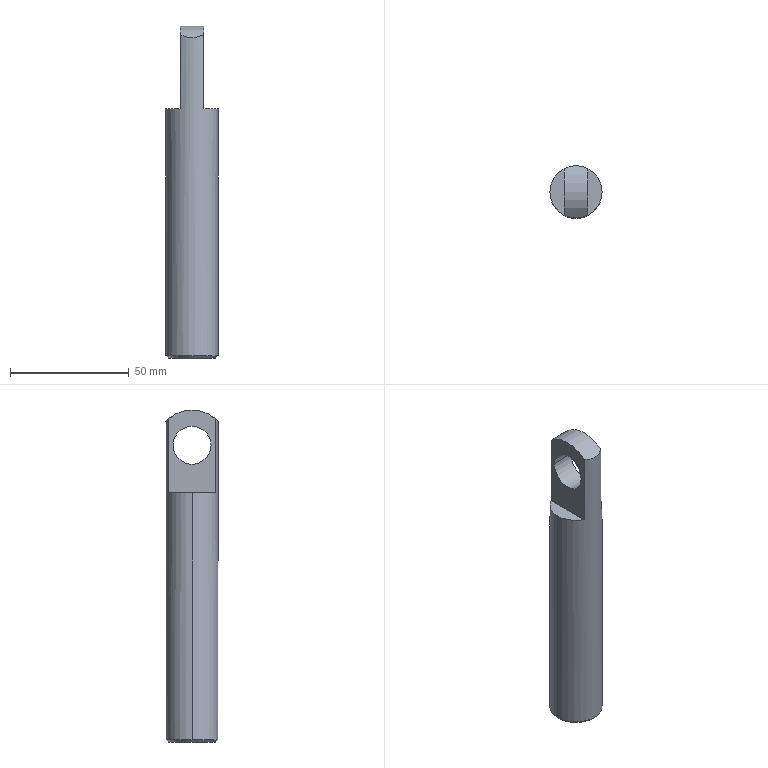Part | SolidWorks | features ICE 2, 3DProfileFeature 1, Chamfer 1, Extrusion 1, HoleWzd 1 | 1 solid | 16 faces | box 22 x 22 x 139.866 mm | volume 36266 mm3 | cylinder 7 | plane 5 | cone 4 | commonest cylinder face diameters 10.5 x2 16 x2 22 x2 29.733 x1
STEP:
#1=CARTESIAN_POINT('',(5.,-8.,125.));
#2=VERTEX_POINT('',#1);
#3=CARTESIAN_POINT('',(5.,8.,125.));
#4=VERTEX_POINT('',#3);
#5=CARTESIAN_POINT('',(5.,0.,125.));
#6=DIRECTION('',(1.,0.,0.));
#7=DIRECTION('',(0.,1.,0.));
#8=AXIS2_PLACEMENT_3D('',#5,#6,#7);
#9=CIRCLE('',#8,8.);
#10=EDGE_CURVE('',#2,#4,#9,.T.);
#11=ORIENTED_EDGE('',*,*,#10,.T.);
#12=CARTESIAN_POINT('',(-5.,8.,125.));
#13=VERTEX_POINT('',#12);
#14=CARTESIAN_POINT('',(11.,8.,125.));
#15=DIRECTION('',(-1.,0.,0.));
#16=VECTOR('',#15,1000.);
#17=LINE('',#14,#16);
#18=EDGE_CURVE('',#4,#13,#17,.T.);
#19=ORIENTED_EDGE('',*,*,#18,.T.);
#20=CARTESIAN_POINT('',(-5.,-8.,125.));
#21=VERTEX_POINT('',#20);
#22=CARTESIAN_POINT('',(-5.,0.,125.));
#23=DIRECTION('',(-1.,0.,0.));
#24=DIRECTION('',(0.,-1.,0.));
#25=AXIS2_PLACEMENT_3D('',#22,#23,#24);
#26=CIRCLE('',#25,8.);
#27=EDGE_CURVE('',#13,#21,#26,.T.);
#28=ORIENTED_EDGE('',*,*,#27,.T.);
#29=CARTESIAN_POINT('',(11.,-8.,125.));
#30=DIRECTION('',(-1.,0.,0.));
#31=VECTOR('',#30,1000.);
#32=LINE('',#29,#31);
#33=EDGE_CURVE('',#2,#21,#32,.T.);
#34=ORIENTED_EDGE('',*,*,#33,.F.);
#35=EDGE_LOOP('',(#11,#19,#28,#34));
#36=FACE_OUTER_BOUND('',#35,.T.);
#37=CARTESIAN_POINT('',(11.,0.,125.));
#38=DIRECTION('',(-1.,0.,0.));
#39=DIRECTION('',(0.,-1.,0.));
#40=AXIS2_PLACEMENT_3D('',#37,#38,#39);
#41=CYLINDRICAL_SURFACE('',#40,8.);
#42=ADVANCED_FACE('',(#36),#41,.F.);
#43=CARTESIAN_POINT('',(-10.,0.,0.));
#44=VERTEX_POINT('',#43);
#45=CARTESIAN_POINT('',(10.,0.,0.));
#46=VERTEX_POINT('',#45);
#47=CARTESIAN_POINT('',(0.,0.,0.));
#48=DIRECTION('',(0.,0.,-1.));
#49=DIRECTION('',(1.,0.,0.));
#50=AXIS2_PLACEMENT_3D('',#47,#48,#49);
#51=CIRCLE('',#50,10.);
#52=EDGE_CURVE('',#44,#46,#51,.T.);
#53=ORIENTED_EDGE('',*,*,#52,.F.);
#54=CARTESIAN_POINT('',(-11.,0.,1.));
#55=VERTEX_POINT('',#54);
#56=CARTESIAN_POINT('',(-11.,0.,1.));
#57=DIRECTION('',(-0.7071,0.,0.7071));
#58=VECTOR('',#57,1000.);
#59=LINE('',#56,#58);
#60=EDGE_CURVE('',#44,#55,#59,.T.);
#61=ORIENTED_EDGE('',*,*,#60,.T.);
#62=CARTESIAN_POINT('',(11.,0.,1.));
#63=VERTEX_POINT('',#62);
#64=CARTESIAN_POINT('',(0.,0.,1.));
#65=DIRECTION('',(0.,0.,1.));
#66=DIRECTION('',(1.,0.,0.));
#67=AXIS2_PLACEMENT_3D('',#64,#65,#66);
#68=CIRCLE('',#67,11.);
#69=EDGE_CURVE('',#63,#55,#68,.T.);
#70=ORIENTED_EDGE('',*,*,#69,.F.);
#71=CARTESIAN_POINT('',(11.,0.,1.));
#72=DIRECTION('',(0.7071,0.,0.7071));
#73=VECTOR('',#72,1000.);
#74=LINE('',#71,#73);
#75=EDGE_CURVE('',#46,#63,#74,.T.);
#76=ORIENTED_EDGE('',*,*,#75,.F.);
#77=EDGE_LOOP('',(#53,#61,#70,#76));
#78=FACE_OUTER_BOUND('',#77,.T.);
#79=CARTESIAN_POINT('',(0.,0.,1.));
#80=DIRECTION('',(0.,0.,1.));
#81=DIRECTION('',(1.,0.,0.));
#82=AXIS2_PLACEMENT_3D('',#79,#80,#81);
#83=CONICAL_SURFACE('',#82,11.,0.7854);
#84=ADVANCED_FACE('',(#78),#83,.T.);
#85=CARTESIAN_POINT('',(5.25,-0.0003502,99.5));
#86=VERTEX_POINT('',#85);
#87=CARTESIAN_POINT('',(-5.25,-0.0003502,99.5));
#88=VERTEX_POINT('',#87);
#89=CARTESIAN_POINT('',(-0.0002667,-0.0003502,99.5));
#90=DIRECTION('',(0.,0.,-1.));
#91=DIRECTION('',(-1.,0.,0.));
#92=AXIS2_PLACEMENT_3D('',#89,#90,#91);
#93=CIRCLE('',#92,5.25);
#94=EDGE_CURVE('',#86,#88,#93,.T.);
#95=ORIENTED_EDGE('',*,*,#94,.F.);
#96=CARTESIAN_POINT('',(5.25,-0.0003502,0.));
#97=VERTEX_POINT('',#96);
#98=CARTESIAN_POINT('',(5.25,-0.0003502,0.));
#99=DIRECTION('',(0.,0.,-1.));
#100=VECTOR('',#99,1000.);
#101=LINE('',#98,#100);
#102=EDGE_CURVE('',#86,#97,#101,.T.);
#103=ORIENTED_EDGE('',*,*,#102,.T.);
#104=CARTESIAN_POINT('',(-5.25,-0.0003502,0.));
#105=VERTEX_POINT('',#104);
#106=CARTESIAN_POINT('',(-0.0002667,-0.0003502,0.));
#107=DIRECTION('',(0.,0.,-1.));
#108=DIRECTION('',(-1.,0.,0.));
#109=AXIS2_PLACEMENT_3D('',#106,#107,#108);
#110=CIRCLE('',#109,5.25);
#111=EDGE_CURVE('',#97,#105,#110,.T.);
#112=ORIENTED_EDGE('',*,*,#111,.T.);
#113=CARTESIAN_POINT('',(-5.25,-0.0003502,0.));
#114=DIRECTION('',(0.,0.,-1.));
#115=VECTOR('',#114,1000.);
#116=LINE('',#113,#115);
#117=EDGE_CURVE('',#88,#105,#116,.T.);
#118=ORIENTED_EDGE('',*,*,#117,.F.);
#119=EDGE_LOOP('',(#95,#103,#112,#118));
#120=FACE_OUTER_BOUND('',#119,.T.);
#121=CARTESIAN_POINT('',(-0.0002667,-0.0003502,0.));
#122=DIRECTION('',(0.,0.,-1.));
#123=DIRECTION('',(-1.,0.,0.));
#124=AXIS2_PLACEMENT_3D('',#121,#122,#123);
#125=CYLINDRICAL_SURFACE('',#124,5.25);
#126=ADVANCED_FACE('',(#120),#125,.F.);
#127=CARTESIAN_POINT('',(-0.0002667,-0.0003502,102.655));
#128=VERTEX_POINT('',#127);
#129=CARTESIAN_POINT('',(-5.25,-0.0003502,99.5));
#130=DIRECTION('',(-0.8572,0.,-0.515));
#131=VECTOR('',#130,1000.);
#132=LINE('',#129,#131);
#133=EDGE_CURVE('',#128,#88,#132,.T.);
#134=ORIENTED_EDGE('',*,*,#133,.F.);
#135=CARTESIAN_POINT('',(5.25,-0.0003502,99.5));
#136=DIRECTION('',(0.8572,0.,-0.515));
#137=VECTOR('',#136,1000.);
#138=LINE('',#135,#137);
#139=EDGE_CURVE('',#128,#86,#138,.T.);
#140=ORIENTED_EDGE('',*,*,#139,.T.);
#141=ORIENTED_EDGE('',*,*,#94,.T.);
#142=EDGE_LOOP('',(#134,#140,#141));
#143=FACE_OUTER_BOUND('',#142,.T.);
#144=CARTESIAN_POINT('',(-0.0002667,-0.0003502,99.5));
#145=DIRECTION('',(0.,0.,-1.));
#146=DIRECTION('',(-1.,0.,0.));
#147=AXIS2_PLACEMENT_3D('',#144,#145,#146);
#148=CONICAL_SURFACE('',#147,5.25,1.03);
#149=ADVANCED_FACE('',(#143),#148,.F.);
#150=CARTESIAN_POINT('',(11.,0.,105.));
#151=VERTEX_POINT('',#150);
#152=CARTESIAN_POINT('',(5.,9.798,105.));
#153=VERTEX_POINT('',#152);
#154=CARTESIAN_POINT('',(0.,0.,105.));
#155=DIRECTION('',(0.,0.,1.));
#156=DIRECTION('',(1.,0.,0.));
#157=AXIS2_PLACEMENT_3D('',#154,#155,#156);
#158=CIRCLE('',#157,11.);
#159=EDGE_CURVE('',#151,#153,#158,.T.);
#160=ORIENTED_EDGE('',*,*,#159,.F.);
#161=CARTESIAN_POINT('',(11.,0.,140.));
#162=DIRECTION('',(0.,0.,-1.));
#163=VECTOR('',#162,1000.);
#164=LINE('',#161,#163);
#165=EDGE_CURVE('',#151,#63,#164,.T.);
#166=ORIENTED_EDGE('',*,*,#165,.T.);
#167=ORIENTED_EDGE('',*,*,#69,.T.);
#168=CARTESIAN_POINT('',(-11.,0.,105.));
#169=VERTEX_POINT('',#168);
#170=CARTESIAN_POINT('',(-11.,0.,140.));
#171=DIRECTION('',(0.,0.,-1.));
#172=VECTOR('',#171,1000.);
#173=LINE('',#170,#172);
#174=EDGE_CURVE('',#169,#55,#173,.T.);
#175=ORIENTED_EDGE('',*,*,#174,.F.);
#176=CARTESIAN_POINT('',(-5.,9.798,105.));
#177=VERTEX_POINT('',#176);
#178=CARTESIAN_POINT('',(0.,0.,105.));
#179=DIRECTION('',(0.,0.,1.));
#180=DIRECTION('',(1.,0.,0.));
#181=AXIS2_PLACEMENT_3D('',#178,#179,#180);
#182=CIRCLE('',#181,11.);
#183=EDGE_CURVE('',#177,#169,#182,.T.);
#184=ORIENTED_EDGE('',*,*,#183,.F.);
#185=CARTESIAN_POINT('',(-5.,9.798,136.181));
#186=VERTEX_POINT('',#185);
#187=CARTESIAN_POINT('',(-5.,9.798,140.));
#188=DIRECTION('',(0.,0.,-1.));
#189=VECTOR('',#188,1000.);
#190=LINE('',#187,#189);
#191=EDGE_CURVE('',#186,#177,#190,.T.);
#192=ORIENTED_EDGE('',*,*,#191,.F.);
#193=CARTESIAN_POINT('',(5.,9.798,136.181));
#194=VERTEX_POINT('',#193);
#195=CARTESIAN_POINT('',(-5.,9.798,136.181));
#196=CARTESIAN_POINT('',(-4.256,10.178,135.848));
#197=CARTESIAN_POINT('',(-3.469,10.475,135.554));
#198=CARTESIAN_POINT('',(-2.412,10.735,135.285));
#199=CARTESIAN_POINT('',(-2.196,10.781,135.237));
#200=CARTESIAN_POINT('',(-1.764,10.86,135.153));
#201=CARTESIAN_POINT('',(-1.547,10.893,135.117));
#202=CARTESIAN_POINT('',(-0.8918,10.973,135.031));
#203=CARTESIAN_POINT('',(-0.4511,11.,135.001));
#204=CARTESIAN_POINT('',(0.4396,11.,135.));
#205=CARTESIAN_POINT('',(0.8929,10.973,135.031));
#206=CARTESIAN_POINT('',(1.772,10.865,135.147));
#207=CARTESIAN_POINT('',(2.202,10.786,135.232));
#208=CARTESIAN_POINT('',(3.046,10.579,135.446));
#209=CARTESIAN_POINT('',(3.46,10.45,135.576));
#210=CARTESIAN_POINT('',(4.252,10.154,135.861));
#211=CARTESIAN_POINT('',(4.632,9.986,136.017));
#212=CARTESIAN_POINT('',(5.,9.798,136.181));
#213=B_SPLINE_CURVE_WITH_KNOTS('',3,(#195,#196,#197,#198,#199,#200,#201,#202,#203,#204,#205,#206,#207,#208,#209,#210,#211,#212),.UNSPECIFIED.,.F.,.F.,(4,2,2,2,2,2,2,2,4),(0.,0.002672,0.00334,0.004008,0.005344,0.00668,0.008015,0.009351,0.01069),.UNSPECIFIED.);
#214=EDGE_CURVE('',#186,#194,#213,.T.);
#215=ORIENTED_EDGE('',*,*,#214,.T.);
#216=CARTESIAN_POINT('',(5.,9.798,140.));
#217=DIRECTION('',(0.,0.,1.));
#218=VECTOR('',#217,1000.);
#219=LINE('',#216,#218);
#220=EDGE_CURVE('',#153,#194,#219,.T.);
#221=ORIENTED_EDGE('',*,*,#220,.F.);
#222=EDGE_LOOP('',(#160,#166,#167,#175,#184,#192,#215,#221));
#223=FACE_OUTER_BOUND('',#222,.T.);
#224=CARTESIAN_POINT('',(0.,0.,140.));
#225=DIRECTION('',(0.,0.,-1.));
#226=DIRECTION('',(-1.,0.,0.));
#227=AXIS2_PLACEMENT_3D('',#224,#225,#226);
#228=CYLINDRICAL_SURFACE('',#227,11.);
#229=ADVANCED_FACE('',(#223),#228,.T.);
#230=ORIENTED_EDGE('',*,*,#165,.F.);
#231=CARTESIAN_POINT('',(5.,-9.798,105.));
#232=VERTEX_POINT('',#231);
#233=CARTESIAN_POINT('',(0.,0.,105.));
#234=DIRECTION('',(0.,0.,1.));
#235=DIRECTION('',(1.,0.,0.));
#236=AXIS2_PLACEMENT_3D('',#233,#234,#235);
#237=CIRCLE('',#236,11.);
#238=EDGE_CURVE('',#232,#151,#237,.T.);
#239=ORIENTED_EDGE('',*,*,#238,.F.);
#240=CARTESIAN_POINT('',(5.,-9.798,136.181));
#241=VERTEX_POINT('',#240);
#242=CARTESIAN_POINT('',(5.,-9.798,140.));
#243=DIRECTION('',(0.,0.,-1.));
#244=VECTOR('',#243,1000.);
#245=LINE('',#242,#244);
#246=EDGE_CURVE('',#241,#232,#245,.T.);
#247=ORIENTED_EDGE('',*,*,#246,.F.);
#248=CARTESIAN_POINT('',(-5.,-9.798,136.181));
#249=VERTEX_POINT('',#248);
#250=CARTESIAN_POINT('',(5.,-9.798,136.181));
#251=CARTESIAN_POINT('',(4.632,-9.986,136.016));
#252=CARTESIAN_POINT('',(4.246,-10.156,135.858));
#253=CARTESIAN_POINT('',(3.453,-10.453,135.573));
#254=CARTESIAN_POINT('',(3.046,-10.579,135.446));
#255=CARTESIAN_POINT('',(2.417,-10.733,135.287));
#256=CARTESIAN_POINT('',(2.205,-10.779,135.239));
#257=CARTESIAN_POINT('',(1.773,-10.858,135.154));
#258=CARTESIAN_POINT('',(1.553,-10.892,135.118));
#259=CARTESIAN_POINT('',(0.891,-10.973,135.031));
#260=CARTESIAN_POINT('',(0.4493,-11.,135.001));
#261=CARTESIAN_POINT('',(-0.4348,-11.,135.));
#262=CARTESIAN_POINT('',(-0.8771,-10.974,135.029));
#263=CARTESIAN_POINT('',(-1.762,-10.867,135.145));
#264=CARTESIAN_POINT('',(-2.195,-10.787,135.231));
#265=CARTESIAN_POINT('',(-3.456,-10.479,135.55));
#266=CARTESIAN_POINT('',(-4.256,-10.178,135.848));
#267=CARTESIAN_POINT('',(-5.,-9.798,136.181));
#268=B_SPLINE_CURVE_WITH_KNOTS('',3,(#250,#251,#252,#253,#254,#255,#256,#257,#258,#259,#260,#261,#262,#263,#264,#265,#266,#267),.UNSPECIFIED.,.F.,.F.,(4,2,2,2,2,2,2,2,4),(0.03612,0.03745,0.03878,0.03945,0.04011,0.04144,0.04278,0.04411,0.04677),.UNSPECIFIED.);
#269=EDGE_CURVE('',#241,#249,#268,.T.);
#270=ORIENTED_EDGE('',*,*,#269,.T.);
#271=CARTESIAN_POINT('',(-5.,-9.798,105.));
#272=VERTEX_POINT('',#271);
#273=CARTESIAN_POINT('',(-5.,-9.798,140.));
#274=DIRECTION('',(0.,0.,1.));
#275=VECTOR('',#274,1000.);
#276=LINE('',#273,#275);
#277=EDGE_CURVE('',#272,#249,#276,.T.);
#278=ORIENTED_EDGE('',*,*,#277,.F.);
#279=CARTESIAN_POINT('',(0.,0.,105.));
#280=DIRECTION('',(0.,0.,1.));
#281=DIRECTION('',(1.,0.,0.));
#282=AXIS2_PLACEMENT_3D('',#279,#280,#281);
#283=CIRCLE('',#282,11.);
#284=EDGE_CURVE('',#169,#272,#283,.T.);
#285=ORIENTED_EDGE('',*,*,#284,.F.);
#286=ORIENTED_EDGE('',*,*,#174,.T.);
#287=CARTESIAN_POINT('',(0.,0.,1.));
#288=DIRECTION('',(0.,0.,1.));
#289=DIRECTION('',(1.,0.,0.));
#290=AXIS2_PLACEMENT_3D('',#287,#288,#289);
#291=CIRCLE('',#290,11.);
#292=EDGE_CURVE('',#55,#63,#291,.T.);
#293=ORIENTED_EDGE('',*,*,#292,.T.);
#294=EDGE_LOOP('',(#230,#239,#247,#270,#278,#285,#286,#293));
#295=FACE_OUTER_BOUND('',#294,.T.);
#296=CARTESIAN_POINT('',(0.,0.,140.));
#297=DIRECTION('',(0.,0.,-1.));
#298=DIRECTION('',(-1.,0.,0.));
#299=AXIS2_PLACEMENT_3D('',#296,#297,#298);
#300=CYLINDRICAL_SURFACE('',#299,11.);
#301=ADVANCED_FACE('',(#295),#300,.T.);
#302=CARTESIAN_POINT('',(0.,0.,0.));
#303=DIRECTION('',(0.,0.,-1.));
#304=DIRECTION('',(1.,0.,0.));
#305=AXIS2_PLACEMENT_3D('',#302,#303,#304);
#306=CIRCLE('',#305,10.);
#307=EDGE_CURVE('',#46,#44,#306,.T.);
#308=ORIENTED_EDGE('',*,*,#307,.T.);
#309=ORIENTED_EDGE('',*,*,#52,.T.);
#310=EDGE_LOOP('',(#308,#309));
#311=FACE_OUTER_BOUND('',#310,.T.);
#312=CARTESIAN_POINT('',(-0.0002667,-0.0003502,0.));
#313=DIRECTION('',(0.,0.,-1.));
#314=DIRECTION('',(-1.,0.,0.));
#315=AXIS2_PLACEMENT_3D('',#312,#313,#314);
#316=CIRCLE('',#315,5.25);
#317=EDGE_CURVE('',#105,#97,#316,.T.);
#318=ORIENTED_EDGE('',*,*,#317,.F.);
#319=ORIENTED_EDGE('',*,*,#111,.F.);
#320=EDGE_LOOP('',(#318,#319));
#321=FACE_BOUND('',#320,.T.);
#322=CARTESIAN_POINT('',(0.,0.,0.));
#323=DIRECTION('',(0.,0.,1.));
#324=DIRECTION('',(1.,0.,0.));
#325=AXIS2_PLACEMENT_3D('',#322,#323,#324);
#326=PLANE('',#325);
#327=ADVANCED_FACE('',(#311,#321),#326,.F.);
#328=ORIENTED_EDGE('',*,*,#183,.T.);
#329=ORIENTED_EDGE('',*,*,#284,.T.);
#330=CARTESIAN_POINT('',(-5.,14.687,105.));
#331=DIRECTION('',(0.,1.,0.));
#332=VECTOR('',#331,1000.);
#333=LINE('',#330,#332);
#334=EDGE_CURVE('',#272,#177,#333,.T.);
#335=ORIENTED_EDGE('',*,*,#334,.T.);
#336=EDGE_LOOP('',(#328,#329,#335));
#337=FACE_OUTER_BOUND('',#336,.T.);
#338=CARTESIAN_POINT('',(0.,0.,105.));
#339=DIRECTION('',(0.,0.,1.));
#340=DIRECTION('',(1.,0.,0.));
#341=AXIS2_PLACEMENT_3D('',#338,#339,#340);
#342=PLANE('',#341);
#343=ADVANCED_FACE('',(#337),#342,.T.);
#344=CARTESIAN_POINT('',(-5.,0.,125.));
#345=DIRECTION('',(1.,0.,0.));
#346=DIRECTION('',(0.,-1.,0.));
#347=AXIS2_PLACEMENT_3D('',#344,#345,#346);
#348=CIRCLE('',#347,14.866);
#349=EDGE_CURVE('',#186,#249,#348,.T.);
#350=ORIENTED_EDGE('',*,*,#349,.F.);
#351=ORIENTED_EDGE('',*,*,#191,.T.);
#352=ORIENTED_EDGE('',*,*,#334,.F.);
#353=ORIENTED_EDGE('',*,*,#277,.T.);
#354=EDGE_LOOP('',(#350,#351,#352,#353));
#355=FACE_OUTER_BOUND('',#354,.T.);
#356=CARTESIAN_POINT('',(-5.,0.,125.));
#357=DIRECTION('',(-1.,0.,0.));
#358=DIRECTION('',(0.,-1.,0.));
#359=AXIS2_PLACEMENT_3D('',#356,#357,#358);
#360=CIRCLE('',#359,8.);
#361=EDGE_CURVE('',#21,#13,#360,.T.);
#362=ORIENTED_EDGE('',*,*,#361,.F.);
#363=ORIENTED_EDGE('',*,*,#27,.F.);
#364=EDGE_LOOP('',(#362,#363));
#365=FACE_BOUND('',#364,.T.);
#366=CARTESIAN_POINT('',(-5.,14.687,140.));
#367=DIRECTION('',(-1.,0.,0.));
#368=DIRECTION('',(0.,-1.,0.));
#369=AXIS2_PLACEMENT_3D('',#366,#367,#368);
#370=PLANE('',#369);
#371=ADVANCED_FACE('',(#355,#365),#370,.T.);
#372=ORIENTED_EDGE('',*,*,#238,.T.);
#373=ORIENTED_EDGE('',*,*,#159,.T.);
#374=CARTESIAN_POINT('',(5.,14.349,105.));
#375=DIRECTION('',(0.,-1.,0.));
#376=VECTOR('',#375,1000.);
#377=LINE('',#374,#376);
#378=EDGE_CURVE('',#153,#232,#377,.T.);
#379=ORIENTED_EDGE('',*,*,#378,.T.);
#380=EDGE_LOOP('',(#372,#373,#379));
#381=FACE_OUTER_BOUND('',#380,.T.);
#382=CARTESIAN_POINT('',(0.,0.,105.));
#383=DIRECTION('',(0.,0.,1.));
#384=DIRECTION('',(1.,0.,0.));
#385=AXIS2_PLACEMENT_3D('',#382,#383,#384);
#386=PLANE('',#385);
#387=ADVANCED_FACE('',(#381),#386,.T.);
#388=CARTESIAN_POINT('',(5.,0.,125.));
#389=DIRECTION('',(-1.,0.,0.));
#390=DIRECTION('',(0.,1.,0.));
#391=AXIS2_PLACEMENT_3D('',#388,#389,#390);
#392=CIRCLE('',#391,14.866);
#393=EDGE_CURVE('',#241,#194,#392,.T.);
#394=ORIENTED_EDGE('',*,*,#393,.F.);
#395=ORIENTED_EDGE('',*,*,#246,.T.);
#396=ORIENTED_EDGE('',*,*,#378,.F.);
#397=ORIENTED_EDGE('',*,*,#220,.T.);
#398=EDGE_LOOP('',(#394,#395,#396,#397));
#399=FACE_OUTER_BOUND('',#398,.T.);
#400=ORIENTED_EDGE('',*,*,#10,.F.);
#401=CARTESIAN_POINT('',(5.,0.,125.));
#402=DIRECTION('',(1.,0.,0.));
#403=DIRECTION('',(0.,1.,0.));
#404=AXIS2_PLACEMENT_3D('',#401,#402,#403);
#405=CIRCLE('',#404,8.);
#406=EDGE_CURVE('',#4,#2,#405,.T.);
#407=ORIENTED_EDGE('',*,*,#406,.F.);
#408=EDGE_LOOP('',(#400,#407));
#409=FACE_BOUND('',#408,.T.);
#410=CARTESIAN_POINT('',(5.,14.349,140.));
#411=DIRECTION('',(1.,0.,0.));
#412=DIRECTION('',(0.,1.,0.));
#413=AXIS2_PLACEMENT_3D('',#410,#411,#412);
#414=PLANE('',#413);
#415=ADVANCED_FACE('',(#399,#409),#414,.T.);
#416=ORIENTED_EDGE('',*,*,#139,.F.);
#417=ORIENTED_EDGE('',*,*,#133,.T.);
#418=CARTESIAN_POINT('',(-0.0002667,-0.0003502,99.5));
#419=DIRECTION('',(0.,0.,-1.));
#420=DIRECTION('',(-1.,0.,0.));
#421=AXIS2_PLACEMENT_3D('',#418,#419,#420);
#422=CIRCLE('',#421,5.25);
#423=EDGE_CURVE('',#88,#86,#422,.T.);
#424=ORIENTED_EDGE('',*,*,#423,.T.);
#425=EDGE_LOOP('',(#416,#417,#424));
#426=FACE_OUTER_BOUND('',#425,.T.);
#427=CARTESIAN_POINT('',(-0.0002667,-0.0003502,99.5));
#428=DIRECTION('',(0.,0.,-1.));
#429=DIRECTION('',(-1.,0.,0.));
#430=AXIS2_PLACEMENT_3D('',#427,#428,#429);
#431=CONICAL_SURFACE('',#430,5.25,1.03);
#432=ADVANCED_FACE('',(#426),#431,.F.);
#433=ORIENTED_EDGE('',*,*,#102,.F.);
#434=ORIENTED_EDGE('',*,*,#423,.F.);
#435=ORIENTED_EDGE('',*,*,#117,.T.);
#436=ORIENTED_EDGE('',*,*,#317,.T.);
#437=EDGE_LOOP('',(#433,#434,#435,#436));
#438=FACE_OUTER_BOUND('',#437,.T.);
#439=CARTESIAN_POINT('',(-0.0002667,-0.0003502,0.));
#440=DIRECTION('',(0.,0.,-1.));
#441=DIRECTION('',(-1.,0.,0.));
#442=AXIS2_PLACEMENT_3D('',#439,#440,#441);
#443=CYLINDRICAL_SURFACE('',#442,5.25);
#444=ADVANCED_FACE('',(#438),#443,.F.);
#445=ORIENTED_EDGE('',*,*,#60,.F.);
#446=ORIENTED_EDGE('',*,*,#307,.F.);
#447=ORIENTED_EDGE('',*,*,#75,.T.);
#448=ORIENTED_EDGE('',*,*,#292,.F.);
#449=EDGE_LOOP('',(#445,#446,#447,#448));
#450=FACE_OUTER_BOUND('',#449,.T.);
#451=CARTESIAN_POINT('',(0.,0.,1.));
#452=DIRECTION('',(0.,0.,1.));
#453=DIRECTION('',(1.,0.,0.));
#454=AXIS2_PLACEMENT_3D('',#451,#452,#453);
#455=CONICAL_SURFACE('',#454,11.,0.7854);
#456=ADVANCED_FACE('',(#450),#455,.T.);
#457=ORIENTED_EDGE('',*,*,#18,.F.);
#458=ORIENTED_EDGE('',*,*,#406,.T.);
#459=ORIENTED_EDGE('',*,*,#33,.T.);
#460=ORIENTED_EDGE('',*,*,#361,.T.);
#461=EDGE_LOOP('',(#457,#458,#459,#460));
#462=FACE_OUTER_BOUND('',#461,.T.);
#463=CARTESIAN_POINT('',(11.,0.,125.));
#464=DIRECTION('',(-1.,0.,0.));
#465=DIRECTION('',(0.,-1.,0.));
#466=AXIS2_PLACEMENT_3D('',#463,#464,#465);
#467=CYLINDRICAL_SURFACE('',#466,8.);
#468=ADVANCED_FACE('',(#462),#467,.F.);
#469=ORIENTED_EDGE('',*,*,#349,.T.);
#470=ORIENTED_EDGE('',*,*,#269,.F.);
#471=ORIENTED_EDGE('',*,*,#393,.T.);
#472=ORIENTED_EDGE('',*,*,#214,.F.);
#473=EDGE_LOOP('',(#469,#470,#471,#472));
#474=FACE_OUTER_BOUND('',#473,.T.);
#475=CARTESIAN_POINT('',(11.,0.,125.));
#476=DIRECTION('',(-1.,0.,0.));
#477=DIRECTION('',(0.,-1.,0.));
#478=AXIS2_PLACEMENT_3D('',#475,#476,#477);
#479=CYLINDRICAL_SURFACE('',#478,14.866);
#480=ADVANCED_FACE('',(#474),#479,.T.);
#481=CLOSED_SHELL('',(#42,#84,#126,#149,#229,#301,#327,#343,#371,#387,#415,#432,#444,#456,#468,#480));
#482=MANIFOLD_SOLID_BREP('',#481);
#483=CARTESIAN_POINT('',(0.,0.,0.));
#484=DIRECTION('',(0.,0.,1.));
#485=DIRECTION('',(1.,0.,0.));
#486=AXIS2_PLACEMENT_3D('',#483,#484,#485);
#487=(LENGTH_UNIT()NAMED_UNIT(*)SI_UNIT(.MILLI.,.METRE.));
#488=UNCERTAINTY_MEASURE_WITH_UNIT(LENGTH_MEASURE(0.00001),#487,'','');
#489=(NAMED_UNIT(*)PLANE_ANGLE_UNIT()SI_UNIT($,.RADIAN.));
#490=(NAMED_UNIT(*)SI_UNIT($,.STERADIAN.)SOLID_ANGLE_UNIT());
#491=(GEOMETRIC_REPRESENTATION_CONTEXT(3)GLOBAL_UNCERTAINTY_ASSIGNED_CONTEXT((#488))GLOBAL_UNIT_ASSIGNED_CONTEXT((#487,#489,#490))REPRESENTATION_CONTEXT('',''));
#492=ADVANCED_BREP_SHAPE_REPRESENTATION('',(#482,#486),#491);